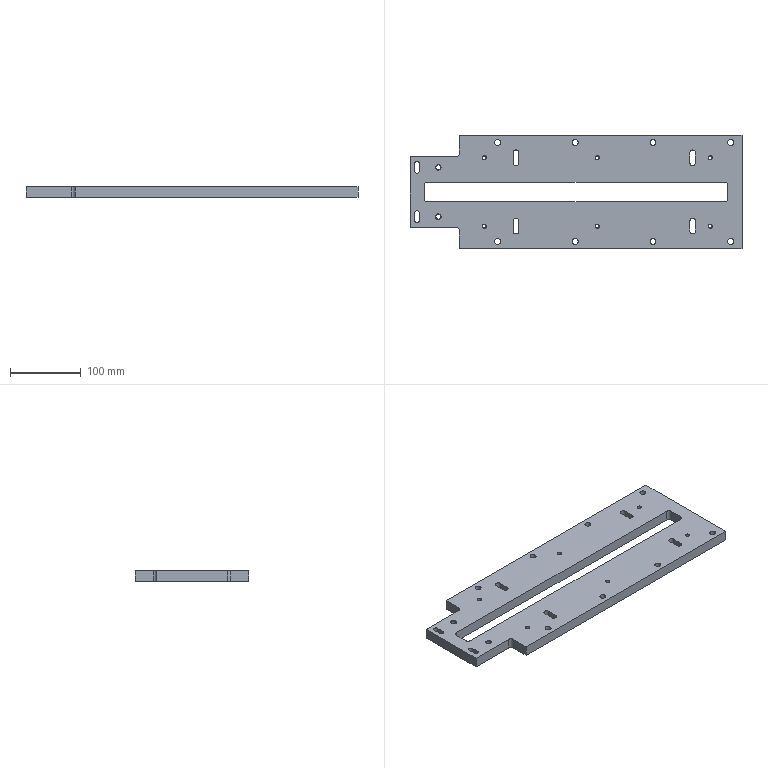Part | STEP file | Tube feed_id658_x_t | 1 solid | 76 faces | box 470 x 160 x 15 mm | volume 862310 mm3 | cylinder 34 | plane 26 | cone 16 | commonest cylinder face diameters 8 x8 8.5 x8 5 x6 6.8 x6 10 x6